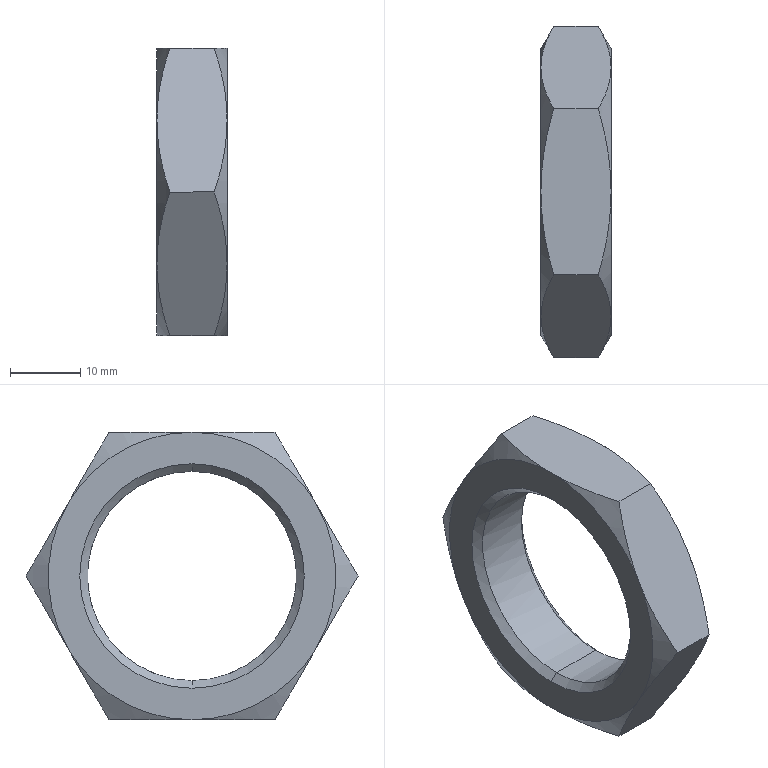Part | SolidWorks | features BaseBody 1 | 1 solid | 26 faces | box 10 x 47.343 x 41 mm | volume 7305 mm3 | cone 16 | plane 8 | cylinder 2 | commonest cylinder face diameters 29.835 x2
STEP:
#1=CARTESIAN_POINT('',(1.083,0.,14.918));
#2=VERTEX_POINT('',#1);
#3=CARTESIAN_POINT('',(1.083,0.,-14.918));
#4=VERTEX_POINT('',#3);
#5=CARTESIAN_POINT('',(1.083,0.,0.));
#6=DIRECTION('',(1.,0.,0.));
#7=DIRECTION('',(0.,0.,-1.));
#8=AXIS2_PLACEMENT_3D('',#5,#6,#7);
#9=CIRCLE('',#8,14.918);
#10=EDGE_CURVE('',#2,#4,#9,.T.);
#11=ORIENTED_EDGE('',*,*,#10,.F.);
#12=CARTESIAN_POINT('',(8.918,0.,14.918));
#13=VERTEX_POINT('',#12);
#14=CARTESIAN_POINT('',(10.,0.,14.918));
#15=DIRECTION('',(1.,0.,0.));
#16=VECTOR('',#15,1000.);
#17=LINE('',#14,#16);
#18=EDGE_CURVE('',#2,#13,#17,.T.);
#19=ORIENTED_EDGE('',*,*,#18,.T.);
#20=CARTESIAN_POINT('',(8.918,-14.918,0.));
#21=VERTEX_POINT('',#20);
#22=CARTESIAN_POINT('',(8.918,0.,0.));
#23=DIRECTION('',(-1.,0.,0.));
#24=DIRECTION('',(0.,0.,-1.));
#25=AXIS2_PLACEMENT_3D('',#22,#23,#24);
#26=CIRCLE('',#25,14.918);
#27=EDGE_CURVE('',#21,#13,#26,.T.);
#28=ORIENTED_EDGE('',*,*,#27,.F.);
#29=CARTESIAN_POINT('',(8.918,0.,-14.918));
#30=VERTEX_POINT('',#29);
#31=CARTESIAN_POINT('',(8.918,0.,0.));
#32=DIRECTION('',(-1.,0.,0.));
#33=DIRECTION('',(0.,0.,-1.));
#34=AXIS2_PLACEMENT_3D('',#31,#32,#33);
#35=CIRCLE('',#34,14.918);
#36=EDGE_CURVE('',#30,#21,#35,.T.);
#37=ORIENTED_EDGE('',*,*,#36,.F.);
#38=CARTESIAN_POINT('',(10.,0.,-14.918));
#39=DIRECTION('',(1.,0.,0.));
#40=VECTOR('',#39,1000.);
#41=LINE('',#38,#40);
#42=EDGE_CURVE('',#4,#30,#41,.T.);
#43=ORIENTED_EDGE('',*,*,#42,.F.);
#44=EDGE_LOOP('',(#11,#19,#28,#37,#43));
#45=FACE_OUTER_BOUND('',#44,.T.);
#46=CARTESIAN_POINT('',(10.,0.,0.));
#47=DIRECTION('',(1.,0.,0.));
#48=DIRECTION('',(0.,0.,-1.));
#49=AXIS2_PLACEMENT_3D('',#46,#47,#48);
#50=CYLINDRICAL_SURFACE('',#49,14.918);
#51=ADVANCED_FACE('',(#45),#50,.F.);
#52=ORIENTED_EDGE('',*,*,#10,.T.);
#53=CARTESIAN_POINT('',(0.,0.,-16.));
#54=VERTEX_POINT('',#53);
#55=CARTESIAN_POINT('',(0.,0.,-16.));
#56=DIRECTION('',(-0.7071,0.,-0.7071));
#57=VECTOR('',#56,1000.);
#58=LINE('',#55,#57);
#59=EDGE_CURVE('',#4,#54,#58,.T.);
#60=ORIENTED_EDGE('',*,*,#59,.T.);
#61=CARTESIAN_POINT('',(0.,0.,16.));
#62=VERTEX_POINT('',#61);
#63=CARTESIAN_POINT('',(0.,0.,0.));
#64=DIRECTION('',(1.,0.,0.));
#65=DIRECTION('',(0.,0.,1.));
#66=AXIS2_PLACEMENT_3D('',#63,#64,#65);
#67=CIRCLE('',#66,16.);
#68=EDGE_CURVE('',#62,#54,#67,.T.);
#69=ORIENTED_EDGE('',*,*,#68,.F.);
#70=CARTESIAN_POINT('',(0.,0.,16.));
#71=DIRECTION('',(-0.7071,0.,0.7071));
#72=VECTOR('',#71,1000.);
#73=LINE('',#70,#72);
#74=EDGE_CURVE('',#2,#62,#73,.T.);
#75=ORIENTED_EDGE('',*,*,#74,.F.);
#76=EDGE_LOOP('',(#52,#60,#69,#75));
#77=FACE_OUTER_BOUND('',#76,.T.);
#78=CARTESIAN_POINT('',(0.,0.,0.));
#79=DIRECTION('',(-1.,0.,0.));
#80=DIRECTION('',(0.,0.,1.));
#81=AXIS2_PLACEMENT_3D('',#78,#79,#80);
#82=CONICAL_SURFACE('',#81,16.,0.7854);
#83=ADVANCED_FACE('',(#77),#82,.F.);
#84=CARTESIAN_POINT('',(8.918,14.918,0.));
#85=VERTEX_POINT('',#84);
#86=CARTESIAN_POINT('',(8.918,0.,0.));
#87=DIRECTION('',(-1.,0.,0.));
#88=DIRECTION('',(0.,0.,-1.));
#89=AXIS2_PLACEMENT_3D('',#86,#87,#88);
#90=CIRCLE('',#89,14.918);
#91=EDGE_CURVE('',#85,#30,#90,.T.);
#92=ORIENTED_EDGE('',*,*,#91,.T.);
#93=ORIENTED_EDGE('',*,*,#36,.T.);
#94=CARTESIAN_POINT('',(10.,-16.,0.));
#95=VERTEX_POINT('',#94);
#96=CARTESIAN_POINT('',(10.,-16.,0.));
#97=DIRECTION('',(0.7071,-0.7071,0.));
#98=VECTOR('',#97,1000.);
#99=LINE('',#96,#98);
#100=EDGE_CURVE('',#21,#95,#99,.T.);
#101=ORIENTED_EDGE('',*,*,#100,.T.);
#102=CARTESIAN_POINT('',(10.,16.,0.));
#103=VERTEX_POINT('',#102);
#104=CARTESIAN_POINT('',(10.,0.,0.));
#105=DIRECTION('',(-1.,0.,0.));
#106=DIRECTION('',(0.,1.,0.));
#107=AXIS2_PLACEMENT_3D('',#104,#105,#106);
#108=CIRCLE('',#107,16.);
#109=EDGE_CURVE('',#103,#95,#108,.T.);
#110=ORIENTED_EDGE('',*,*,#109,.F.);
#111=CARTESIAN_POINT('',(10.,16.,0.));
#112=DIRECTION('',(0.7071,0.7071,0.));
#113=VECTOR('',#112,1000.);
#114=LINE('',#111,#113);
#115=EDGE_CURVE('',#85,#103,#114,.T.);
#116=ORIENTED_EDGE('',*,*,#115,.F.);
#117=EDGE_LOOP('',(#92,#93,#101,#110,#116));
#118=FACE_OUTER_BOUND('',#117,.T.);
#119=CARTESIAN_POINT('',(10.,0.,0.));
#120=DIRECTION('',(1.,0.,0.));
#121=DIRECTION('',(0.,1.,0.));
#122=AXIS2_PLACEMENT_3D('',#119,#120,#121);
#123=CONICAL_SURFACE('',#122,16.,0.7854);
#124=ADVANCED_FACE('',(#118),#123,.F.);
#125=ORIENTED_EDGE('',*,*,#18,.F.);
#126=CARTESIAN_POINT('',(1.083,0.,0.));
#127=DIRECTION('',(1.,0.,0.));
#128=DIRECTION('',(0.,0.,-1.));
#129=AXIS2_PLACEMENT_3D('',#126,#127,#128);
#130=CIRCLE('',#129,14.918);
#131=EDGE_CURVE('',#4,#2,#130,.T.);
#132=ORIENTED_EDGE('',*,*,#131,.F.);
#133=ORIENTED_EDGE('',*,*,#42,.T.);
#134=ORIENTED_EDGE('',*,*,#91,.F.);
#135=CARTESIAN_POINT('',(8.918,0.,0.));
#136=DIRECTION('',(-1.,0.,0.));
#137=DIRECTION('',(0.,0.,-1.));
#138=AXIS2_PLACEMENT_3D('',#135,#136,#137);
#139=CIRCLE('',#138,14.918);
#140=EDGE_CURVE('',#13,#85,#139,.T.);
#141=ORIENTED_EDGE('',*,*,#140,.F.);
#142=EDGE_LOOP('',(#125,#132,#133,#134,#141));
#143=FACE_OUTER_BOUND('',#142,.T.);
#144=CARTESIAN_POINT('',(10.,0.,0.));
#145=DIRECTION('',(1.,0.,0.));
#146=DIRECTION('',(0.,0.,-1.));
#147=AXIS2_PLACEMENT_3D('',#144,#145,#146);
#148=CYLINDRICAL_SURFACE('',#147,14.918);
#149=ADVANCED_FACE('',(#143),#148,.F.);
#150=ORIENTED_EDGE('',*,*,#59,.F.);
#151=ORIENTED_EDGE('',*,*,#131,.T.);
#152=ORIENTED_EDGE('',*,*,#74,.T.);
#153=CARTESIAN_POINT('',(0.,0.,0.));
#154=DIRECTION('',(1.,0.,0.));
#155=DIRECTION('',(0.,0.,1.));
#156=AXIS2_PLACEMENT_3D('',#153,#154,#155);
#157=CIRCLE('',#156,16.);
#158=EDGE_CURVE('',#54,#62,#157,.T.);
#159=ORIENTED_EDGE('',*,*,#158,.F.);
#160=EDGE_LOOP('',(#150,#151,#152,#159));
#161=FACE_OUTER_BOUND('',#160,.T.);
#162=CARTESIAN_POINT('',(0.,0.,0.));
#163=DIRECTION('',(-1.,0.,0.));
#164=DIRECTION('',(0.,0.,1.));
#165=AXIS2_PLACEMENT_3D('',#162,#163,#164);
#166=CONICAL_SURFACE('',#165,16.,0.7854);
#167=ADVANCED_FACE('',(#161),#166,.F.);
#168=ORIENTED_EDGE('',*,*,#100,.F.);
#169=ORIENTED_EDGE('',*,*,#27,.T.);
#170=ORIENTED_EDGE('',*,*,#140,.T.);
#171=ORIENTED_EDGE('',*,*,#115,.T.);
#172=CARTESIAN_POINT('',(10.,0.,0.));
#173=DIRECTION('',(-1.,0.,0.));
#174=DIRECTION('',(0.,1.,0.));
#175=AXIS2_PLACEMENT_3D('',#172,#173,#174);
#176=CIRCLE('',#175,16.);
#177=EDGE_CURVE('',#95,#103,#176,.T.);
#178=ORIENTED_EDGE('',*,*,#177,.F.);
#179=EDGE_LOOP('',(#168,#169,#170,#171,#178));
#180=FACE_OUTER_BOUND('',#179,.T.);
#181=CARTESIAN_POINT('',(10.,0.,0.));
#182=DIRECTION('',(1.,0.,0.));
#183=DIRECTION('',(0.,1.,0.));
#184=AXIS2_PLACEMENT_3D('',#181,#182,#183);
#185=CONICAL_SURFACE('',#184,16.,0.7854);
#186=ADVANCED_FACE('',(#180),#185,.F.);
#187=ORIENTED_EDGE('',*,*,#68,.T.);
#188=ORIENTED_EDGE('',*,*,#158,.T.);
#189=EDGE_LOOP('',(#187,#188));
#190=FACE_BOUND('',#189,.T.);
#191=CARTESIAN_POINT('',(0.,0.,-20.5));
#192=VERTEX_POINT('',#191);
#193=CARTESIAN_POINT('',(0.,17.754,-10.25));
#194=VERTEX_POINT('',#193);
#195=CARTESIAN_POINT('',(0.,0.,0.));
#196=DIRECTION('',(1.,0.,0.));
#197=DIRECTION('',(0.,0.,-1.));
#198=AXIS2_PLACEMENT_3D('',#195,#196,#197);
#199=CIRCLE('',#198,20.5);
#200=EDGE_CURVE('',#192,#194,#199,.T.);
#201=ORIENTED_EDGE('',*,*,#200,.F.);
#202=CARTESIAN_POINT('',(0.,-17.754,-10.25));
#203=VERTEX_POINT('',#202);
#204=CARTESIAN_POINT('',(0.,0.,0.));
#205=DIRECTION('',(1.,0.,0.));
#206=DIRECTION('',(0.,0.,-1.));
#207=AXIS2_PLACEMENT_3D('',#204,#205,#206);
#208=CIRCLE('',#207,20.5);
#209=EDGE_CURVE('',#203,#192,#208,.T.);
#210=ORIENTED_EDGE('',*,*,#209,.F.);
#211=CARTESIAN_POINT('',(0.,-17.754,10.25));
#212=VERTEX_POINT('',#211);
#213=CARTESIAN_POINT('',(0.,0.,0.));
#214=DIRECTION('',(1.,0.,0.));
#215=DIRECTION('',(0.,0.,-1.));
#216=AXIS2_PLACEMENT_3D('',#213,#214,#215);
#217=CIRCLE('',#216,20.5);
#218=EDGE_CURVE('',#212,#203,#217,.T.);
#219=ORIENTED_EDGE('',*,*,#218,.F.);
#220=CARTESIAN_POINT('',(0.,0.,20.5));
#221=VERTEX_POINT('',#220);
#222=CARTESIAN_POINT('',(0.,0.,0.));
#223=DIRECTION('',(1.,0.,0.));
#224=DIRECTION('',(0.,0.,-1.));
#225=AXIS2_PLACEMENT_3D('',#222,#223,#224);
#226=CIRCLE('',#225,20.5);
#227=EDGE_CURVE('',#221,#212,#226,.T.);
#228=ORIENTED_EDGE('',*,*,#227,.F.);
#229=CARTESIAN_POINT('',(0.,17.754,10.25));
#230=VERTEX_POINT('',#229);
#231=CARTESIAN_POINT('',(0.,0.,0.));
#232=DIRECTION('',(1.,0.,0.));
#233=DIRECTION('',(0.,0.,-1.));
#234=AXIS2_PLACEMENT_3D('',#231,#232,#233);
#235=CIRCLE('',#234,20.5);
#236=EDGE_CURVE('',#230,#221,#235,.T.);
#237=ORIENTED_EDGE('',*,*,#236,.F.);
#238=CARTESIAN_POINT('',(0.,0.,0.));
#239=DIRECTION('',(1.,0.,0.));
#240=DIRECTION('',(0.,0.,-1.));
#241=AXIS2_PLACEMENT_3D('',#238,#239,#240);
#242=CIRCLE('',#241,20.5);
#243=EDGE_CURVE('',#194,#230,#242,.T.);
#244=ORIENTED_EDGE('',*,*,#243,.F.);
#245=EDGE_LOOP('',(#201,#210,#219,#228,#237,#244));
#246=FACE_OUTER_BOUND('',#245,.T.);
#247=CARTESIAN_POINT('',(0.,0.,0.));
#248=DIRECTION('',(1.,0.,0.));
#249=DIRECTION('',(0.,0.,-1.));
#250=AXIS2_PLACEMENT_3D('',#247,#248,#249);
#251=PLANE('',#250);
#252=ADVANCED_FACE('',(#190,#246),#251,.F.);
#253=CARTESIAN_POINT('',(10.,17.754,10.25));
#254=VERTEX_POINT('',#253);
#255=CARTESIAN_POINT('',(10.,17.754,-10.25));
#256=VERTEX_POINT('',#255);
#257=CARTESIAN_POINT('',(10.,0.,0.));
#258=DIRECTION('',(-1.,0.,0.));
#259=DIRECTION('',(0.,0.,1.));
#260=AXIS2_PLACEMENT_3D('',#257,#258,#259);
#261=CIRCLE('',#260,20.5);
#262=EDGE_CURVE('',#254,#256,#261,.T.);
#263=ORIENTED_EDGE('',*,*,#262,.F.);
#264=CARTESIAN_POINT('',(10.,0.,20.5));
#265=VERTEX_POINT('',#264);
#266=CARTESIAN_POINT('',(10.,0.,0.));
#267=DIRECTION('',(-1.,0.,0.));
#268=DIRECTION('',(0.,0.,1.));
#269=AXIS2_PLACEMENT_3D('',#266,#267,#268);
#270=CIRCLE('',#269,20.5);
#271=EDGE_CURVE('',#265,#254,#270,.T.);
#272=ORIENTED_EDGE('',*,*,#271,.F.);
#273=CARTESIAN_POINT('',(10.,-17.754,10.25));
#274=VERTEX_POINT('',#273);
#275=CARTESIAN_POINT('',(10.,0.,0.));
#276=DIRECTION('',(-1.,0.,0.));
#277=DIRECTION('',(0.,0.,1.));
#278=AXIS2_PLACEMENT_3D('',#275,#276,#277);
#279=CIRCLE('',#278,20.5);
#280=EDGE_CURVE('',#274,#265,#279,.T.);
#281=ORIENTED_EDGE('',*,*,#280,.F.);
#282=CARTESIAN_POINT('',(10.,-17.754,-10.25));
#283=VERTEX_POINT('',#282);
#284=CARTESIAN_POINT('',(10.,0.,0.));
#285=DIRECTION('',(-1.,0.,0.));
#286=DIRECTION('',(0.,0.,1.));
#287=AXIS2_PLACEMENT_3D('',#284,#285,#286);
#288=CIRCLE('',#287,20.5);
#289=EDGE_CURVE('',#283,#274,#288,.T.);
#290=ORIENTED_EDGE('',*,*,#289,.F.);
#291=CARTESIAN_POINT('',(10.,0.,-20.5));
#292=VERTEX_POINT('',#291);
#293=CARTESIAN_POINT('',(10.,0.,0.));
#294=DIRECTION('',(-1.,0.,0.));
#295=DIRECTION('',(0.,0.,1.));
#296=AXIS2_PLACEMENT_3D('',#293,#294,#295);
#297=CIRCLE('',#296,20.5);
#298=EDGE_CURVE('',#292,#283,#297,.T.);
#299=ORIENTED_EDGE('',*,*,#298,.F.);
#300=CARTESIAN_POINT('',(10.,0.,0.));
#301=DIRECTION('',(-1.,0.,0.));
#302=DIRECTION('',(0.,0.,1.));
#303=AXIS2_PLACEMENT_3D('',#300,#301,#302);
#304=CIRCLE('',#303,20.5);
#305=EDGE_CURVE('',#256,#292,#304,.T.);
#306=ORIENTED_EDGE('',*,*,#305,.F.);
#307=EDGE_LOOP('',(#263,#272,#281,#290,#299,#306));
#308=FACE_OUTER_BOUND('',#307,.T.);
#309=ORIENTED_EDGE('',*,*,#109,.T.);
#310=ORIENTED_EDGE('',*,*,#177,.T.);
#311=EDGE_LOOP('',(#309,#310));
#312=FACE_BOUND('',#311,.T.);
#313=CARTESIAN_POINT('',(10.,20.5,0.));
#314=DIRECTION('',(-1.,0.,0.));
#315=DIRECTION('',(0.,0.,1.));
#316=AXIS2_PLACEMENT_3D('',#313,#314,#315);
#317=PLANE('',#316);
#318=ADVANCED_FACE('',(#308,#312),#317,.F.);
#319=ORIENTED_EDGE('',*,*,#243,.T.);
#320=CARTESIAN_POINT('',(1.831,23.671,-0.000000014));
#321=VERTEX_POINT('',#320);
#322=CARTESIAN_POINT('',(0.,17.754,10.25));
#323=CARTESIAN_POINT('',(0.,18.763,8.501));
#324=CARTESIAN_POINT('',(0.175,19.76,6.775));
#325=CARTESIAN_POINT('',(0.8125,21.73,3.362));
#326=CARTESIAN_POINT('',(1.273,22.705,1.674));
#327=CARTESIAN_POINT('',(1.831,23.671,-0.000000014));
#328=B_SPLINE_CURVE_WITH_KNOTS('',3,(#322,#323,#324,#325,#326,#327),.UNSPECIFIED.,.F.,.F.,(4,2,4),(0.,0.005988,0.01198),.UNSPECIFIED.);
#329=EDGE_CURVE('',#230,#321,#328,.T.);
#330=ORIENTED_EDGE('',*,*,#329,.T.);
#331=CARTESIAN_POINT('',(1.831,23.671,-0.000000014));
#332=CARTESIAN_POINT('',(1.273,22.705,-1.674));
#333=CARTESIAN_POINT('',(0.8125,21.73,-3.362));
#334=CARTESIAN_POINT('',(0.175,19.76,-6.775));
#335=CARTESIAN_POINT('',(0.,18.763,-8.501));
#336=CARTESIAN_POINT('',(0.,17.754,-10.25));
#337=B_SPLINE_CURVE_WITH_KNOTS('',3,(#331,#332,#333,#334,#335,#336),.UNSPECIFIED.,.F.,.F.,(4,2,4),(0.,0.005988,0.01198),.UNSPECIFIED.);
#338=EDGE_CURVE('',#321,#194,#337,.T.);
#339=ORIENTED_EDGE('',*,*,#338,.T.);
#340=EDGE_LOOP('',(#319,#330,#339));
#341=FACE_OUTER_BOUND('',#340,.T.);
#342=CARTESIAN_POINT('',(1.842,0.,0.));
#343=DIRECTION('',(1.,0.,0.));
#344=DIRECTION('',(0.,0.,-1.));
#345=AXIS2_PLACEMENT_3D('',#342,#343,#344);
#346=CONICAL_SURFACE('',#345,23.69,1.047);
#347=ADVANCED_FACE('',(#341),#346,.T.);
#348=CARTESIAN_POINT('',(1.831,11.836,-20.5));
#349=VERTEX_POINT('',#348);
#350=CARTESIAN_POINT('',(0.,17.754,-10.25));
#351=CARTESIAN_POINT('',(0.,16.744,-11.999));
#352=CARTESIAN_POINT('',(0.175,15.747,-13.725));
#353=CARTESIAN_POINT('',(0.8125,13.777,-17.138));
#354=CARTESIAN_POINT('',(1.273,12.802,-18.826));
#355=CARTESIAN_POINT('',(1.831,11.836,-20.5));
#356=B_SPLINE_CURVE_WITH_KNOTS('',3,(#350,#351,#352,#353,#354,#355),.UNSPECIFIED.,.F.,.F.,(4,2,4),(0.,0.005988,0.01198),.UNSPECIFIED.);
#357=EDGE_CURVE('',#194,#349,#356,.T.);
#358=ORIENTED_EDGE('',*,*,#357,.T.);
#359=CARTESIAN_POINT('',(1.831,11.836,-20.5));
#360=CARTESIAN_POINT('',(1.273,9.902,-20.5));
#361=CARTESIAN_POINT('',(0.8125,7.954,-20.5));
#362=CARTESIAN_POINT('',(0.175,4.013,-20.5));
#363=CARTESIAN_POINT('',(0.,2.02,-20.5));
#364=CARTESIAN_POINT('',(0.,0.,-20.5));
#365=B_SPLINE_CURVE_WITH_KNOTS('',3,(#359,#360,#361,#362,#363,#364),.UNSPECIFIED.,.F.,.F.,(4,2,4),(0.,0.005988,0.01198),.UNSPECIFIED.);
#366=EDGE_CURVE('',#349,#192,#365,.T.);
#367=ORIENTED_EDGE('',*,*,#366,.T.);
#368=ORIENTED_EDGE('',*,*,#200,.T.);
#369=EDGE_LOOP('',(#358,#367,#368));
#370=FACE_OUTER_BOUND('',#369,.T.);
#371=CARTESIAN_POINT('',(1.842,0.,0.));
#372=DIRECTION('',(1.,0.,0.));
#373=DIRECTION('',(0.,0.,-1.));
#374=AXIS2_PLACEMENT_3D('',#371,#372,#373);
#375=CONICAL_SURFACE('',#374,23.69,1.047);
#376=ADVANCED_FACE('',(#370),#375,.T.);
#377=CARTESIAN_POINT('',(1.831,-11.836,-20.5));
#378=VERTEX_POINT('',#377);
#379=CARTESIAN_POINT('',(0.,0.,-20.5));
#380=CARTESIAN_POINT('',(0.,-2.02,-20.5));
#381=CARTESIAN_POINT('',(0.175,-4.013,-20.5));
#382=CARTESIAN_POINT('',(0.8125,-7.954,-20.5));
#383=CARTESIAN_POINT('',(1.273,-9.902,-20.5));
#384=CARTESIAN_POINT('',(1.831,-11.836,-20.5));
#385=B_SPLINE_CURVE_WITH_KNOTS('',3,(#379,#380,#381,#382,#383,#384),.UNSPECIFIED.,.F.,.F.,(4,2,4),(0.,0.005988,0.01198),.UNSPECIFIED.);
#386=EDGE_CURVE('',#192,#378,#385,.T.);
#387=ORIENTED_EDGE('',*,*,#386,.T.);
#388=CARTESIAN_POINT('',(1.831,-11.836,-20.5));
#389=CARTESIAN_POINT('',(1.273,-12.802,-18.826));
#390=CARTESIAN_POINT('',(0.8125,-13.777,-17.138));
#391=CARTESIAN_POINT('',(0.175,-15.747,-13.725));
#392=CARTESIAN_POINT('',(0.,-16.744,-11.999));
#393=CARTESIAN_POINT('',(0.,-17.754,-10.25));
#394=B_SPLINE_CURVE_WITH_KNOTS('',3,(#388,#389,#390,#391,#392,#393),.UNSPECIFIED.,.F.,.F.,(4,2,4),(0.,0.005988,0.01198),.UNSPECIFIED.);
#395=EDGE_CURVE('',#378,#203,#394,.T.);
#396=ORIENTED_EDGE('',*,*,#395,.T.);
#397=ORIENTED_EDGE('',*,*,#209,.T.);
#398=EDGE_LOOP('',(#387,#396,#397));
#399=FACE_OUTER_BOUND('',#398,.T.);
#400=CARTESIAN_POINT('',(1.842,0.,0.));
#401=DIRECTION('',(1.,0.,0.));
#402=DIRECTION('',(0.,0.,-1.));
#403=AXIS2_PLACEMENT_3D('',#400,#401,#402);
#404=CONICAL_SURFACE('',#403,23.69,1.047);
#405=ADVANCED_FACE('',(#399),#404,.T.);
#406=CARTESIAN_POINT('',(1.831,-23.671,-0.000000038));
#407=VERTEX_POINT('',#406);
#408=CARTESIAN_POINT('',(0.,-17.754,-10.25));
#409=CARTESIAN_POINT('',(0.,-18.763,-8.501));
#410=CARTESIAN_POINT('',(0.175,-19.76,-6.775));
#411=CARTESIAN_POINT('',(0.8125,-21.73,-3.362));
#412=CARTESIAN_POINT('',(1.273,-22.705,-1.674));
#413=CARTESIAN_POINT('',(1.831,-23.671,-0.000000038));
#414=B_SPLINE_CURVE_WITH_KNOTS('',3,(#408,#409,#410,#411,#412,#413),.UNSPECIFIED.,.F.,.F.,(4,2,4),(0.,0.005988,0.01198),.UNSPECIFIED.);
#415=EDGE_CURVE('',#203,#407,#414,.T.);
#416=ORIENTED_EDGE('',*,*,#415,.T.);
#417=CARTESIAN_POINT('',(1.831,-23.671,-0.000000038));
#418=CARTESIAN_POINT('',(1.273,-22.705,1.674));
#419=CARTESIAN_POINT('',(0.8125,-21.73,3.362));
#420=CARTESIAN_POINT('',(0.175,-19.76,6.775));
#421=CARTESIAN_POINT('',(0.,-18.763,8.501));
#422=CARTESIAN_POINT('',(0.,-17.754,10.25));
#423=B_SPLINE_CURVE_WITH_KNOTS('',3,(#417,#418,#419,#420,#421,#422),.UNSPECIFIED.,.F.,.F.,(4,2,4),(0.,0.005988,0.01198),.UNSPECIFIED.);
#424=EDGE_CURVE('',#407,#212,#423,.T.);
#425=ORIENTED_EDGE('',*,*,#424,.T.);
#426=ORIENTED_EDGE('',*,*,#218,.T.);
#427=EDGE_LOOP('',(#416,#425,#426));
#428=FACE_OUTER_BOUND('',#427,.T.);
#429=CARTESIAN_POINT('',(1.842,0.,0.));
#430=DIRECTION('',(1.,0.,0.));
#431=DIRECTION('',(0.,0.,-1.));
#432=AXIS2_PLACEMENT_3D('',#429,#430,#431);
#433=CONICAL_SURFACE('',#432,23.69,1.047);
#434=ADVANCED_FACE('',(#428),#433,.T.);
#435=CARTESIAN_POINT('',(1.831,-11.836,20.5));
#436=VERTEX_POINT('',#435);
#437=CARTESIAN_POINT('',(1.831,-11.836,20.5));
#438=CARTESIAN_POINT('',(1.273,-9.902,20.5));
#439=CARTESIAN_POINT('',(0.8125,-7.954,20.5));
#440=CARTESIAN_POINT('',(0.175,-4.013,20.5));
#441=CARTESIAN_POINT('',(0.,-2.02,20.5));
#442=CARTESIAN_POINT('',(0.,0.,20.5));
#443=B_SPLINE_CURVE_WITH_KNOTS('',3,(#437,#438,#439,#440,#441,#442),.UNSPECIFIED.,.F.,.F.,(4,2,4),(0.,0.005988,0.01198),.UNSPECIFIED.);
#444=EDGE_CURVE('',#436,#221,#443,.T.);
#445=ORIENTED_EDGE('',*,*,#444,.T.);
#446=ORIENTED_EDGE('',*,*,#227,.T.);
#447=CARTESIAN_POINT('',(0.,-17.754,10.25));
#448=CARTESIAN_POINT('',(0.,-16.744,11.999));
#449=CARTESIAN_POINT('',(0.175,-15.747,13.725));
#450=CARTESIAN_POINT('',(0.8125,-13.777,17.138));
#451=CARTESIAN_POINT('',(1.273,-12.802,18.826));
#452=CARTESIAN_POINT('',(1.831,-11.836,20.5));
#453=B_SPLINE_CURVE_WITH_KNOTS('',3,(#447,#448,#449,#450,#451,#452),.UNSPECIFIED.,.F.,.F.,(4,2,4),(0.,0.005988,0.01198),.UNSPECIFIED.);
#454=EDGE_CURVE('',#212,#436,#453,.T.);
#455=ORIENTED_EDGE('',*,*,#454,.T.);
#456=EDGE_LOOP('',(#445,#446,#455));
#457=FACE_OUTER_BOUND('',#456,.T.);
#458=CARTESIAN_POINT('',(1.842,0.,0.));
#459=DIRECTION('',(1.,0.,0.));
#460=DIRECTION('',(0.,0.,-1.));
#461=AXIS2_PLACEMENT_3D('',#458,#459,#460);
#462=CONICAL_SURFACE('',#461,23.69,1.047);
#463=ADVANCED_FACE('',(#457),#462,.T.);
#464=CARTESIAN_POINT('',(1.831,11.836,20.5));
#465=VERTEX_POINT('',#464);
#466=CARTESIAN_POINT('',(0.,0.,20.5));
#467=CARTESIAN_POINT('',(0.,2.02,20.5));
#468=CARTESIAN_POINT('',(0.175,4.013,20.5));
#469=CARTESIAN_POINT('',(0.8125,7.954,20.5));
#470=CARTESIAN_POINT('',(1.273,9.902,20.5));
#471=CARTESIAN_POINT('',(1.831,11.836,20.5));
#472=B_SPLINE_CURVE_WITH_KNOTS('',3,(#466,#467,#468,#469,#470,#471),.UNSPECIFIED.,.F.,.F.,(4,2,4),(0.,0.005988,0.01198),.UNSPECIFIED.);
#473=EDGE_CURVE('',#221,#465,#472,.T.);
#474=ORIENTED_EDGE('',*,*,#473,.T.);
#475=CARTESIAN_POINT('',(1.831,11.836,20.5));
#476=CARTESIAN_POINT('',(1.273,12.802,18.826));
#477=CARTESIAN_POINT('',(0.8125,13.777,17.138));
#478=CARTESIAN_POINT('',(0.175,15.747,13.725));
#479=CARTESIAN_POINT('',(0.,16.744,11.999));
#480=CARTESIAN_POINT('',(0.,17.754,10.25));
#481=B_SPLINE_CURVE_WITH_KNOTS('',3,(#475,#476,#477,#478,#479,#480),.UNSPECIFIED.,.F.,.F.,(4,2,4),(0.,0.005988,0.01198),.UNSPECIFIED.);
#482=EDGE_CURVE('',#465,#230,#481,.T.);
#483=ORIENTED_EDGE('',*,*,#482,.T.);
#484=ORIENTED_EDGE('',*,*,#236,.T.);
#485=EDGE_LOOP('',(#474,#483,#484));
#486=FACE_OUTER_BOUND('',#485,.T.);
#487=CARTESIAN_POINT('',(1.842,0.,0.));
#488=DIRECTION('',(1.,0.,0.));
#489=DIRECTION('',(0.,0.,-1.));
#490=AXIS2_PLACEMENT_3D('',#487,#488,#489);
#491=CONICAL_SURFACE('',#490,23.69,1.047);
#492=ADVANCED_FACE('',(#486),#491,.T.);
#493=CARTESIAN_POINT('',(8.169,11.836,-20.5));
#494=VERTEX_POINT('',#493);
#495=CARTESIAN_POINT('',(8.169,11.836,-20.5));
#496=CARTESIAN_POINT('',(8.727,12.802,-18.826));
#497=CARTESIAN_POINT('',(9.187,13.777,-17.138));
#498=CARTESIAN_POINT('',(9.825,15.747,-13.725));
#499=CARTESIAN_POINT('',(10.,16.744,-11.999));
#500=CARTESIAN_POINT('',(10.,17.754,-10.25));
#501=B_SPLINE_CURVE_WITH_KNOTS('',3,(#495,#496,#497,#498,#499,#500),.UNSPECIFIED.,.F.,.F.,(4,2,4),(0.,0.005988,0.01198),.UNSPECIFIED.);
#502=EDGE_CURVE('',#494,#256,#501,.T.);
#503=ORIENTED_EDGE('',*,*,#502,.T.);
#504=ORIENTED_EDGE('',*,*,#305,.T.);
#505=CARTESIAN_POINT('',(10.,0.,-20.5));
#506=CARTESIAN_POINT('',(10.,2.02,-20.5));
#507=CARTESIAN_POINT('',(9.825,4.013,-20.5));
#508=CARTESIAN_POINT('',(9.187,7.954,-20.5));
#509=CARTESIAN_POINT('',(8.727,9.902,-20.5));
#510=CARTESIAN_POINT('',(8.169,11.836,-20.5));
#511=B_SPLINE_CURVE_WITH_KNOTS('',3,(#505,#506,#507,#508,#509,#510),.UNSPECIFIED.,.F.,.F.,(4,2,4),(0.,0.005988,0.01198),.UNSPECIFIED.);
#512=EDGE_CURVE('',#292,#494,#511,.T.);
#513=ORIENTED_EDGE('',*,*,#512,.T.);
#514=EDGE_LOOP('',(#503,#504,#513));
#515=FACE_OUTER_BOUND('',#514,.T.);
#516=CARTESIAN_POINT('',(8.158,0.,0.));
#517=DIRECTION('',(-1.,0.,0.));
#518=DIRECTION('',(0.,0.,1.));
#519=AXIS2_PLACEMENT_3D('',#516,#517,#518);
#520=CONICAL_SURFACE('',#519,23.69,1.047);
#521=ADVANCED_FACE('',(#515),#520,.T.);
#522=CARTESIAN_POINT('',(8.169,23.671,-0.000000038));
#523=VERTEX_POINT('',#522);
#524=CARTESIAN_POINT('',(10.,17.754,-10.25));
#525=CARTESIAN_POINT('',(10.,18.763,-8.501));
#526=CARTESIAN_POINT('',(9.825,19.76,-6.775));
#527=CARTESIAN_POINT('',(9.187,21.73,-3.362));
#528=CARTESIAN_POINT('',(8.727,22.705,-1.674));
#529=CARTESIAN_POINT('',(8.169,23.671,-0.000000038));
#530=B_SPLINE_CURVE_WITH_KNOTS('',3,(#524,#525,#526,#527,#528,#529),.UNSPECIFIED.,.F.,.F.,(4,2,4),(0.,0.005988,0.01198),.UNSPECIFIED.);
#531=EDGE_CURVE('',#256,#523,#530,.T.);
#532=ORIENTED_EDGE('',*,*,#531,.T.);
#533=CARTESIAN_POINT('',(8.169,23.671,-0.000000038));
#534=CARTESIAN_POINT('',(8.727,22.705,1.674));
#535=CARTESIAN_POINT('',(9.187,21.73,3.362));
#536=CARTESIAN_POINT('',(9.825,19.76,6.775));
#537=CARTESIAN_POINT('',(10.,18.763,8.501));
#538=CARTESIAN_POINT('',(10.,17.754,10.25));
#539=B_SPLINE_CURVE_WITH_KNOTS('',3,(#533,#534,#535,#536,#537,#538),.UNSPECIFIED.,.F.,.F.,(4,2,4),(0.,0.005988,0.01198),.UNSPECIFIED.);
#540=EDGE_CURVE('',#523,#254,#539,.T.);
#541=ORIENTED_EDGE('',*,*,#540,.T.);
#542=ORIENTED_EDGE('',*,*,#262,.T.);
#543=EDGE_LOOP('',(#532,#541,#542));
#544=FACE_OUTER_BOUND('',#543,.T.);
#545=CARTESIAN_POINT('',(8.158,0.,0.));
#546=DIRECTION('',(-1.,0.,0.));
#547=DIRECTION('',(0.,0.,1.));
#548=AXIS2_PLACEMENT_3D('',#545,#546,#547);
#549=CONICAL_SURFACE('',#548,23.69,1.047);
#550=ADVANCED_FACE('',(#544),#549,.T.);
#551=CARTESIAN_POINT('',(8.169,11.836,20.5));
#552=VERTEX_POINT('',#551);
#553=CARTESIAN_POINT('',(10.,17.754,10.25));
#554=CARTESIAN_POINT('',(10.,16.744,11.999));
#555=CARTESIAN_POINT('',(9.825,15.747,13.725));
#556=CARTESIAN_POINT('',(9.187,13.777,17.138));
#557=CARTESIAN_POINT('',(8.727,12.802,18.826));
#558=CARTESIAN_POINT('',(8.169,11.836,20.5));
#559=B_SPLINE_CURVE_WITH_KNOTS('',3,(#553,#554,#555,#556,#557,#558),.UNSPECIFIED.,.F.,.F.,(4,2,4),(0.,0.005988,0.01198),.UNSPECIFIED.);
#560=EDGE_CURVE('',#254,#552,#559,.T.);
#561=ORIENTED_EDGE('',*,*,#560,.T.);
#562=CARTESIAN_POINT('',(8.169,11.836,20.5));
#563=CARTESIAN_POINT('',(8.727,9.902,20.5));
#564=CARTESIAN_POINT('',(9.187,7.954,20.5));
#565=CARTESIAN_POINT('',(9.825,4.013,20.5));
#566=CARTESIAN_POINT('',(10.,2.02,20.5));
#567=CARTESIAN_POINT('',(10.,0.,20.5));
#568=B_SPLINE_CURVE_WITH_KNOTS('',3,(#562,#563,#564,#565,#566,#567),.UNSPECIFIED.,.F.,.F.,(4,2,4),(0.,0.005988,0.01198),.UNSPECIFIED.);
#569=EDGE_CURVE('',#552,#265,#568,.T.);
#570=ORIENTED_EDGE('',*,*,#569,.T.);
#571=ORIENTED_EDGE('',*,*,#271,.T.);
#572=EDGE_LOOP('',(#561,#570,#571));
#573=FACE_OUTER_BOUND('',#572,.T.);
#574=CARTESIAN_POINT('',(8.158,0.,0.));
#575=DIRECTION('',(-1.,0.,0.));
#576=DIRECTION('',(0.,0.,1.));
#577=AXIS2_PLACEMENT_3D('',#574,#575,#576);
#578=CONICAL_SURFACE('',#577,23.69,1.047);
#579=ADVANCED_FACE('',(#573),#578,.T.);
#580=CARTESIAN_POINT('',(8.169,-11.836,20.5));
#581=VERTEX_POINT('',#580);
#582=CARTESIAN_POINT('',(10.,0.,20.5));
#583=CARTESIAN_POINT('',(10.,-2.02,20.5));
#584=CARTESIAN_POINT('',(9.825,-4.013,20.5));
#585=CARTESIAN_POINT('',(9.187,-7.954,20.5));
#586=CARTESIAN_POINT('',(8.727,-9.902,20.5));
#587=CARTESIAN_POINT('',(8.169,-11.836,20.5));
#588=B_SPLINE_CURVE_WITH_KNOTS('',3,(#582,#583,#584,#585,#586,#587),.UNSPECIFIED.,.F.,.F.,(4,2,4),(0.,0.005988,0.01198),.UNSPECIFIED.);
#589=EDGE_CURVE('',#265,#581,#588,.T.);
#590=ORIENTED_EDGE('',*,*,#589,.T.);
#591=CARTESIAN_POINT('',(8.169,-11.836,20.5));
#592=CARTESIAN_POINT('',(8.727,-12.802,18.826));
#593=CARTESIAN_POINT('',(9.187,-13.777,17.138));
#594=CARTESIAN_POINT('',(9.825,-15.747,13.725));
#595=CARTESIAN_POINT('',(10.,-16.744,11.999));
#596=CARTESIAN_POINT('',(10.,-17.754,10.25));
#597=B_SPLINE_CURVE_WITH_KNOTS('',3,(#591,#592,#593,#594,#595,#596),.UNSPECIFIED.,.F.,.F.,(4,2,4),(0.,0.005988,0.01198),.UNSPECIFIED.);
#598=EDGE_CURVE('',#581,#274,#597,.T.);
#599=ORIENTED_EDGE('',*,*,#598,.T.);
#600=ORIENTED_EDGE('',*,*,#280,.T.);
#601=EDGE_LOOP('',(#590,#599,#600));
#602=FACE_OUTER_BOUND('',#601,.T.);
#603=CARTESIAN_POINT('',(8.158,0.,0.));
#604=DIRECTION('',(-1.,0.,0.));
#605=DIRECTION('',(0.,0.,1.));
#606=AXIS2_PLACEMENT_3D('',#603,#604,#605);
#607=CONICAL_SURFACE('',#606,23.69,1.047);
#608=ADVANCED_FACE('',(#602),#607,.T.);
#609=CARTESIAN_POINT('',(8.169,-23.671,0.000000038));
#610=VERTEX_POINT('',#609);
#611=CARTESIAN_POINT('',(8.169,-23.671,0.000000038));
#612=CARTESIAN_POINT('',(8.727,-22.705,-1.674));
#613=CARTESIAN_POINT('',(9.187,-21.73,-3.362));
#614=CARTESIAN_POINT('',(9.825,-19.76,-6.775));
#615=CARTESIAN_POINT('',(10.,-18.763,-8.501));
#616=CARTESIAN_POINT('',(10.,-17.754,-10.25));
#617=B_SPLINE_CURVE_WITH_KNOTS('',3,(#611,#612,#613,#614,#615,#616),.UNSPECIFIED.,.F.,.F.,(4,2,4),(0.,0.005988,0.01198),.UNSPECIFIED.);
#618=EDGE_CURVE('',#610,#283,#617,.T.);
#619=ORIENTED_EDGE('',*,*,#618,.T.);
#620=ORIENTED_EDGE('',*,*,#289,.T.);
#621=CARTESIAN_POINT('',(10.,-17.754,10.25));
#622=CARTESIAN_POINT('',(10.,-18.763,8.501));
#623=CARTESIAN_POINT('',(9.825,-19.76,6.775));
#624=CARTESIAN_POINT('',(9.187,-21.73,3.362));
#625=CARTESIAN_POINT('',(8.727,-22.705,1.674));
#626=CARTESIAN_POINT('',(8.169,-23.671,0.000000038));
#627=B_SPLINE_CURVE_WITH_KNOTS('',3,(#621,#622,#623,#624,#625,#626),.UNSPECIFIED.,.F.,.F.,(4,2,4),(0.,0.005988,0.01198),.UNSPECIFIED.);
#628=EDGE_CURVE('',#274,#610,#627,.T.);
#629=ORIENTED_EDGE('',*,*,#628,.T.);
#630=EDGE_LOOP('',(#619,#620,#629));
#631=FACE_OUTER_BOUND('',#630,.T.);
#632=CARTESIAN_POINT('',(8.158,0.,0.));
#633=DIRECTION('',(-1.,0.,0.));
#634=DIRECTION('',(0.,0.,1.));
#635=AXIS2_PLACEMENT_3D('',#632,#633,#634);
#636=CONICAL_SURFACE('',#635,23.69,1.047);
#637=ADVANCED_FACE('',(#631),#636,.T.);
#638=CARTESIAN_POINT('',(8.169,-11.836,-20.5));
#639=VERTEX_POINT('',#638);
#640=CARTESIAN_POINT('',(8.169,-11.836,-20.5));
#641=CARTESIAN_POINT('',(8.727,-9.902,-20.5));
#642=CARTESIAN_POINT('',(9.187,-7.954,-20.5));
#643=CARTESIAN_POINT('',(9.825,-4.013,-20.5));
#644=CARTESIAN_POINT('',(10.,-2.02,-20.5));
#645=CARTESIAN_POINT('',(10.,0.,-20.5));
#646=B_SPLINE_CURVE_WITH_KNOTS('',3,(#640,#641,#642,#643,#644,#645),.UNSPECIFIED.,.F.,.F.,(4,2,4),(0.,0.005988,0.01198),.UNSPECIFIED.);
#647=EDGE_CURVE('',#639,#292,#646,.T.);
#648=ORIENTED_EDGE('',*,*,#647,.T.);
#649=ORIENTED_EDGE('',*,*,#298,.T.);
#650=CARTESIAN_POINT('',(10.,-17.754,-10.25));
#651=CARTESIAN_POINT('',(10.,-16.744,-11.999));
#652=CARTESIAN_POINT('',(9.825,-15.747,-13.725));
#653=CARTESIAN_POINT('',(9.187,-13.777,-17.138));
#654=CARTESIAN_POINT('',(8.727,-12.802,-18.826));
#655=CARTESIAN_POINT('',(8.169,-11.836,-20.5));
#656=B_SPLINE_CURVE_WITH_KNOTS('',3,(#650,#651,#652,#653,#654,#655),.UNSPECIFIED.,.F.,.F.,(4,2,4),(0.,0.005988,0.01198),.UNSPECIFIED.);
#657=EDGE_CURVE('',#283,#639,#656,.T.);
#658=ORIENTED_EDGE('',*,*,#657,.T.);
#659=EDGE_LOOP('',(#648,#649,#658));
#660=FACE_OUTER_BOUND('',#659,.T.);
#661=CARTESIAN_POINT('',(8.158,0.,0.));
#662=DIRECTION('',(-1.,0.,0.));
#663=DIRECTION('',(0.,0.,1.));
#664=AXIS2_PLACEMENT_3D('',#661,#662,#663);
#665=CONICAL_SURFACE('',#664,23.69,1.047);
#666=ADVANCED_FACE('',(#660),#665,.T.);
#667=ORIENTED_EDGE('',*,*,#560,.F.);
#668=ORIENTED_EDGE('',*,*,#540,.F.);
#669=CARTESIAN_POINT('',(10.,23.671,0.));
#670=DIRECTION('',(1.,0.,0.));
#671=VECTOR('',#670,1000.);
#672=LINE('',#669,#671);
#673=EDGE_CURVE('',#321,#523,#672,.T.);
#674=ORIENTED_EDGE('',*,*,#673,.F.);
#675=ORIENTED_EDGE('',*,*,#329,.F.);
#676=ORIENTED_EDGE('',*,*,#482,.F.);
#677=CARTESIAN_POINT('',(10.,11.836,20.5));
#678=DIRECTION('',(-1.,0.,0.));
#679=VECTOR('',#678,1000.);
#680=LINE('',#677,#679);
#681=EDGE_CURVE('',#552,#465,#680,.T.);
#682=ORIENTED_EDGE('',*,*,#681,.F.);
#683=EDGE_LOOP('',(#667,#668,#674,#675,#676,#682));
#684=FACE_OUTER_BOUND('',#683,.T.);
#685=CARTESIAN_POINT('',(10.,23.671,0.));
#686=DIRECTION('',(0.,-0.866,-0.5));
#687=DIRECTION('',(0.,0.5,-0.866));
#688=AXIS2_PLACEMENT_3D('',#685,#686,#687);
#689=PLANE('',#688);
#690=ADVANCED_FACE('',(#684),#689,.F.);
#691=ORIENTED_EDGE('',*,*,#531,.F.);
#692=ORIENTED_EDGE('',*,*,#502,.F.);
#693=CARTESIAN_POINT('',(10.,11.836,-20.5));
#694=DIRECTION('',(1.,0.,0.));
#695=VECTOR('',#694,1000.);
#696=LINE('',#693,#695);
#697=EDGE_CURVE('',#349,#494,#696,.T.);
#698=ORIENTED_EDGE('',*,*,#697,.F.);
#699=ORIENTED_EDGE('',*,*,#357,.F.);
#700=ORIENTED_EDGE('',*,*,#338,.F.);
#701=ORIENTED_EDGE('',*,*,#673,.T.);
#702=EDGE_LOOP('',(#691,#692,#698,#699,#700,#701));
#703=FACE_OUTER_BOUND('',#702,.T.);
#704=CARTESIAN_POINT('',(10.,11.836,-20.5));
#705=DIRECTION('',(0.,-0.866,0.5));
#706=DIRECTION('',(0.,-0.5,-0.866));
#707=AXIS2_PLACEMENT_3D('',#704,#705,#706);
#708=PLANE('',#707);
#709=ADVANCED_FACE('',(#703),#708,.F.);
#710=ORIENTED_EDGE('',*,*,#512,.F.);
#711=ORIENTED_EDGE('',*,*,#647,.F.);
#712=CARTESIAN_POINT('',(10.,-11.836,-20.5));
#713=DIRECTION('',(1.,0.,0.));
#714=VECTOR('',#713,1000.);
#715=LINE('',#712,#714);
#716=EDGE_CURVE('',#378,#639,#715,.T.);
#717=ORIENTED_EDGE('',*,*,#716,.F.);
#718=ORIENTED_EDGE('',*,*,#386,.F.);
#719=ORIENTED_EDGE('',*,*,#366,.F.);
#720=ORIENTED_EDGE('',*,*,#697,.T.);
#721=EDGE_LOOP('',(#710,#711,#717,#718,#719,#720));
#722=FACE_OUTER_BOUND('',#721,.T.);
#723=CARTESIAN_POINT('',(10.,-11.836,-20.5));
#724=DIRECTION('',(0.,0.,1.));
#725=DIRECTION('',(1.,0.,0.));
#726=AXIS2_PLACEMENT_3D('',#723,#724,#725);
#727=PLANE('',#726);
#728=ADVANCED_FACE('',(#722),#727,.F.);
#729=ORIENTED_EDGE('',*,*,#657,.F.);
#730=ORIENTED_EDGE('',*,*,#618,.F.);
#731=CARTESIAN_POINT('',(10.,-23.671,0.));
#732=DIRECTION('',(1.,0.,0.));
#733=VECTOR('',#732,1000.);
#734=LINE('',#731,#733);
#735=EDGE_CURVE('',#407,#610,#734,.T.);
#736=ORIENTED_EDGE('',*,*,#735,.F.);
#737=ORIENTED_EDGE('',*,*,#415,.F.);
#738=ORIENTED_EDGE('',*,*,#395,.F.);
#739=ORIENTED_EDGE('',*,*,#716,.T.);
#740=EDGE_LOOP('',(#729,#730,#736,#737,#738,#739));
#741=FACE_OUTER_BOUND('',#740,.T.);
#742=CARTESIAN_POINT('',(10.,-23.671,0.));
#743=DIRECTION('',(0.,0.866,0.5));
#744=DIRECTION('',(0.,-0.5,0.866));
#745=AXIS2_PLACEMENT_3D('',#742,#743,#744);
#746=PLANE('',#745);
#747=ADVANCED_FACE('',(#741),#746,.F.);
#748=ORIENTED_EDGE('',*,*,#628,.F.);
#749=ORIENTED_EDGE('',*,*,#598,.F.);
#750=CARTESIAN_POINT('',(10.,-11.836,20.5));
#751=DIRECTION('',(1.,0.,0.));
#752=VECTOR('',#751,1000.);
#753=LINE('',#750,#752);
#754=EDGE_CURVE('',#436,#581,#753,.T.);
#755=ORIENTED_EDGE('',*,*,#754,.F.);
#756=ORIENTED_EDGE('',*,*,#454,.F.);
#757=ORIENTED_EDGE('',*,*,#424,.F.);
#758=ORIENTED_EDGE('',*,*,#735,.T.);
#759=EDGE_LOOP('',(#748,#749,#755,#756,#757,#758));
#760=FACE_OUTER_BOUND('',#759,.T.);
#761=CARTESIAN_POINT('',(10.,-11.836,20.5));
#762=DIRECTION('',(0.,0.866,-0.5));
#763=DIRECTION('',(0.,0.5,0.866));
#764=AXIS2_PLACEMENT_3D('',#761,#762,#763);
#765=PLANE('',#764);
#766=ADVANCED_FACE('',(#760),#765,.F.);
#767=ORIENTED_EDGE('',*,*,#589,.F.);
#768=ORIENTED_EDGE('',*,*,#569,.F.);
#769=ORIENTED_EDGE('',*,*,#681,.T.);
#770=ORIENTED_EDGE('',*,*,#473,.F.);
#771=ORIENTED_EDGE('',*,*,#444,.F.);
#772=ORIENTED_EDGE('',*,*,#754,.T.);
#773=EDGE_LOOP('',(#767,#768,#769,#770,#771,#772));
#774=FACE_OUTER_BOUND('',#773,.T.);
#775=CARTESIAN_POINT('',(10.,11.836,20.5));
#776=DIRECTION('',(0.,0.,-1.));
#777=DIRECTION('',(-1.,0.,0.));
#778=AXIS2_PLACEMENT_3D('',#775,#776,#777);
#779=PLANE('',#778);
#780=ADVANCED_FACE('',(#774),#779,.F.);
#781=CLOSED_SHELL('',(#51,#83,#124,#149,#167,#186,#252,#318,#347,#376,#405,#434,#463,#492,#521,#550,#579,#608,#637,#666,#690,#709,#728,#747,#766,#780));
#782=MANIFOLD_SOLID_BREP('',#781);
#783=CARTESIAN_POINT('',(0.,0.,0.));
#784=DIRECTION('',(0.,0.,1.));
#785=DIRECTION('',(1.,0.,0.));
#786=AXIS2_PLACEMENT_3D('',#783,#784,#785);
#787=(LENGTH_UNIT()NAMED_UNIT(*)SI_UNIT(.MILLI.,.METRE.));
#788=UNCERTAINTY_MEASURE_WITH_UNIT(LENGTH_MEASURE(0.00001),#787,'','');
#789=(NAMED_UNIT(*)PLANE_ANGLE_UNIT()SI_UNIT($,.RADIAN.));
#790=(NAMED_UNIT(*)SI_UNIT($,.STERADIAN.)SOLID_ANGLE_UNIT());
#791=(GEOMETRIC_REPRESENTATION_CONTEXT(3)GLOBAL_UNCERTAINTY_ASSIGNED_CONTEXT((#788))GLOBAL_UNIT_ASSIGNED_CONTEXT((#787,#789,#790))REPRESENTATION_CONTEXT('',''));
#792=ADVANCED_BREP_SHAPE_REPRESENTATION('',(#782,#786),#791);